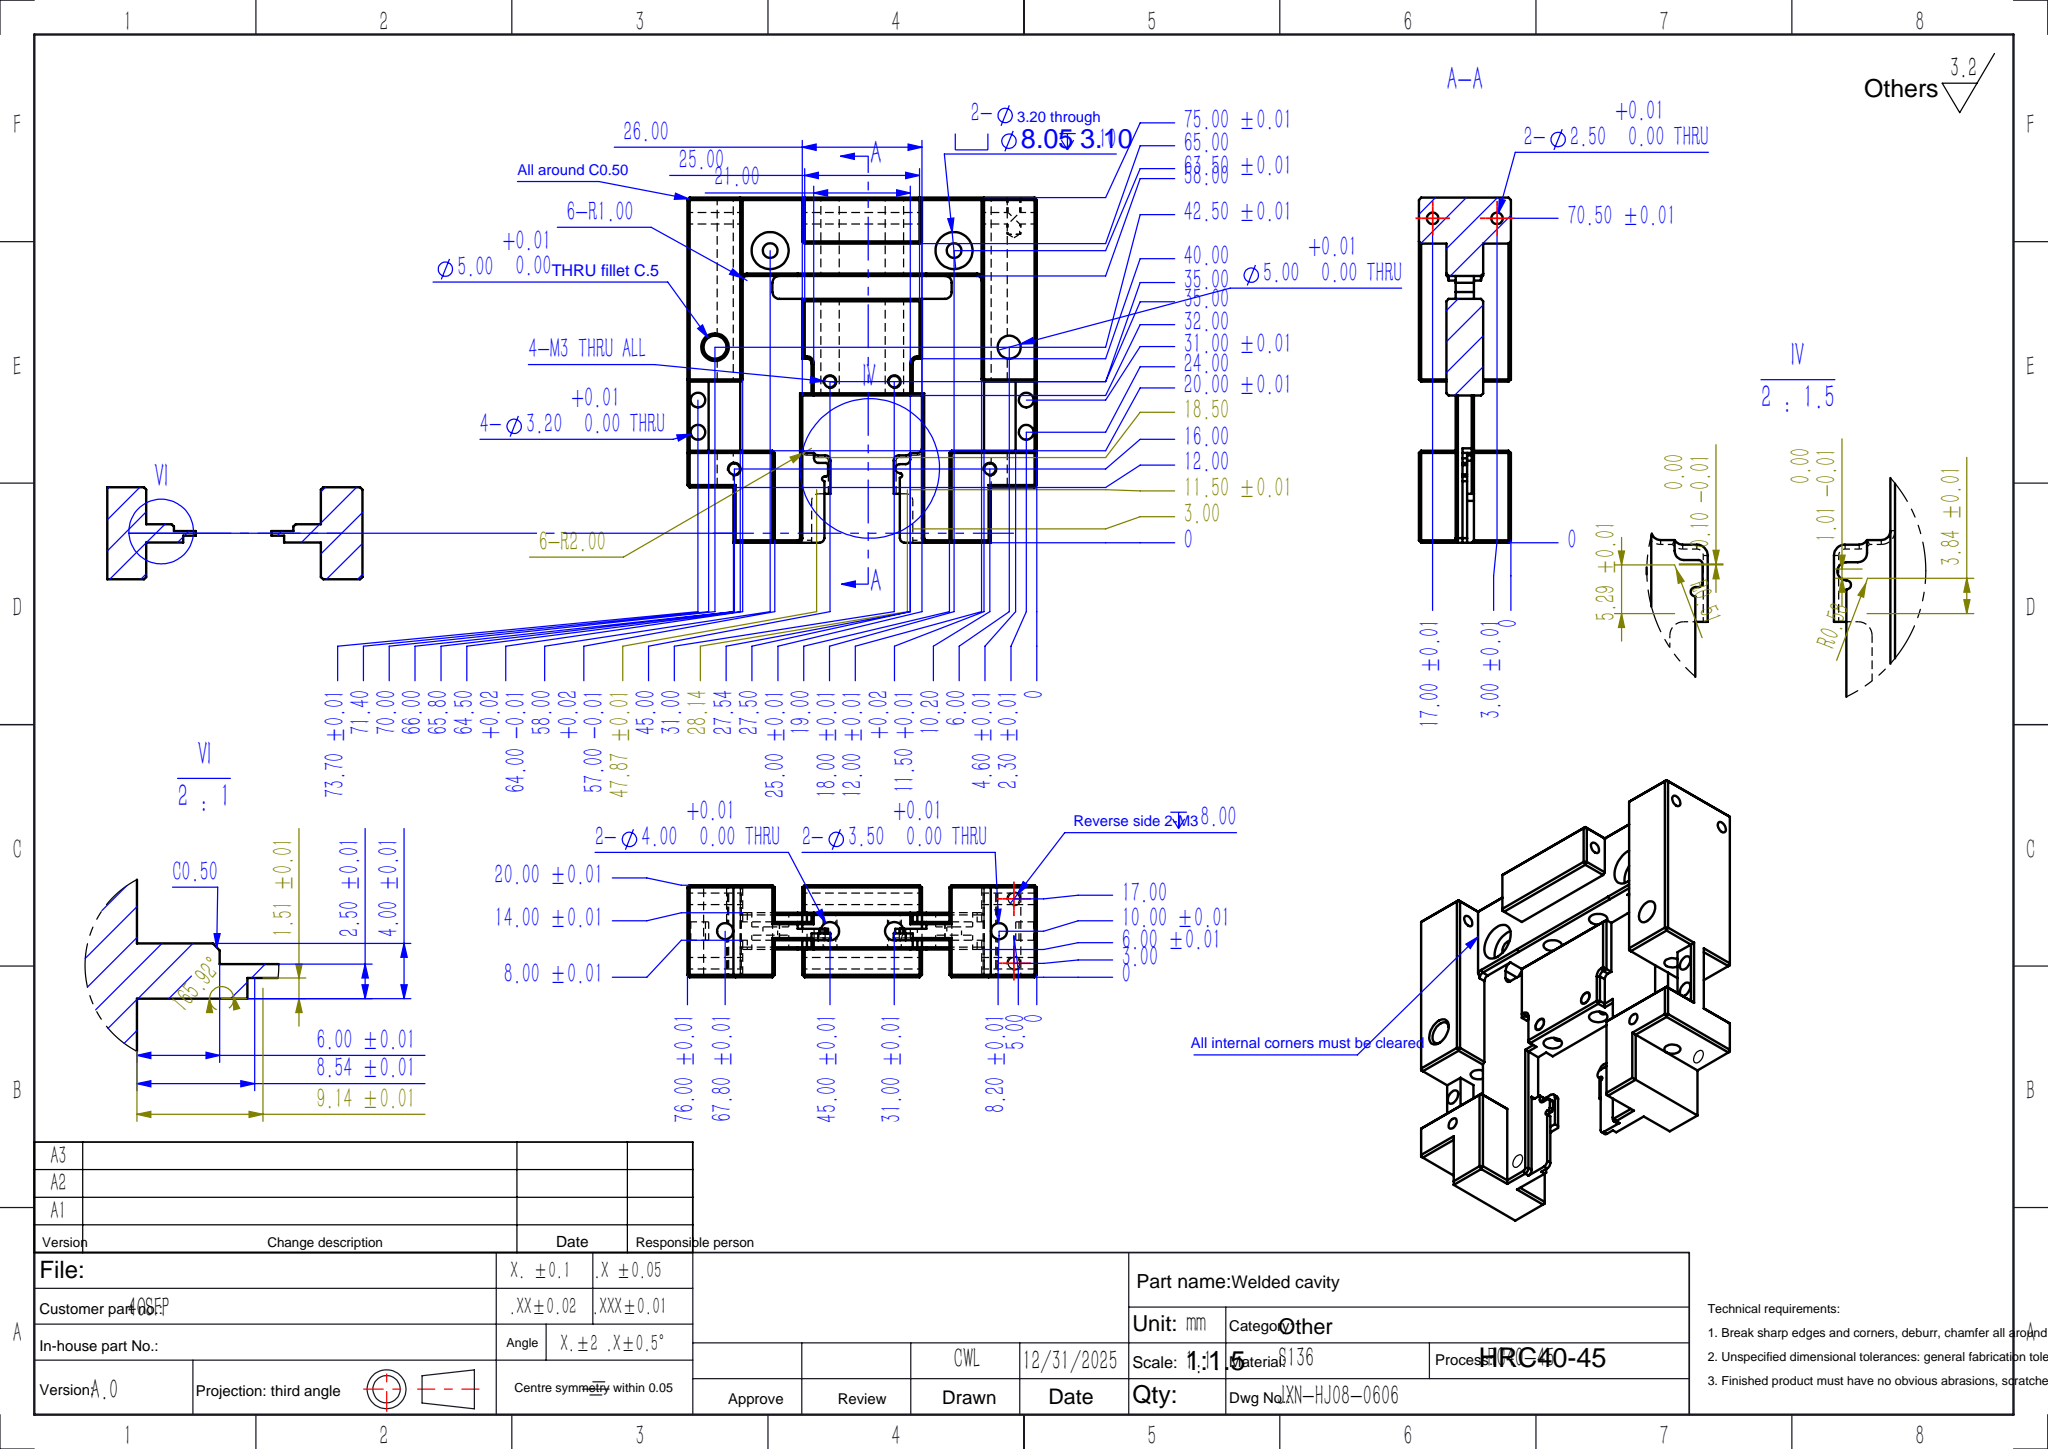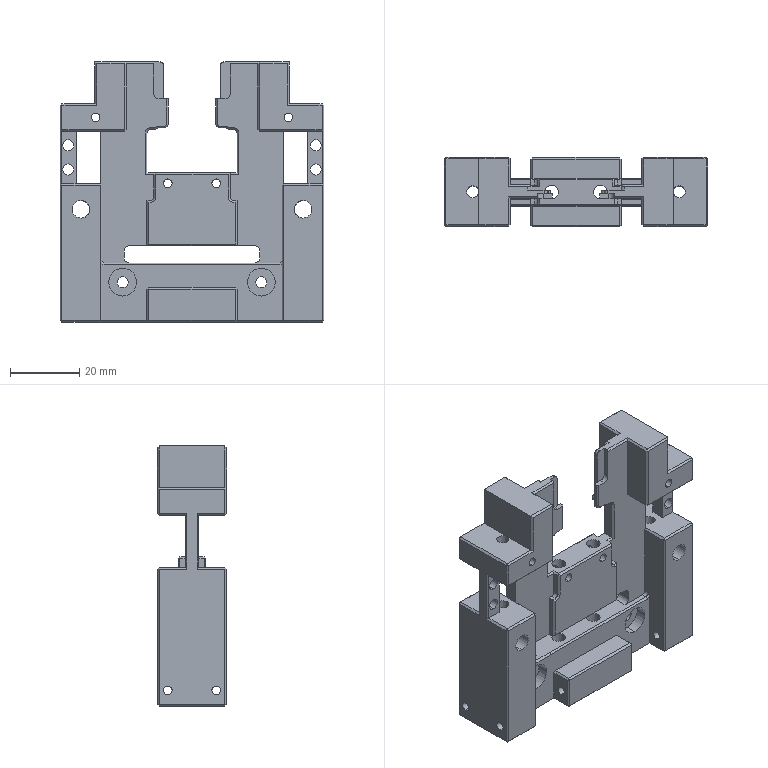Part | SolidWorks | features ICE 34, Fillet 3, HoleWzd 3, Chamfer 2, Cut 2, Extrusion 1 | 1 solid | 408 faces | box 76 x 20 x 75 mm | volume 45299 mm3 | plane 279 | cylinder 107 | cone 22 | commonest cylinder face diameters 2.5 x36 2 x18 3.2 x12 3.5 x8 4 x8 8.05 x8